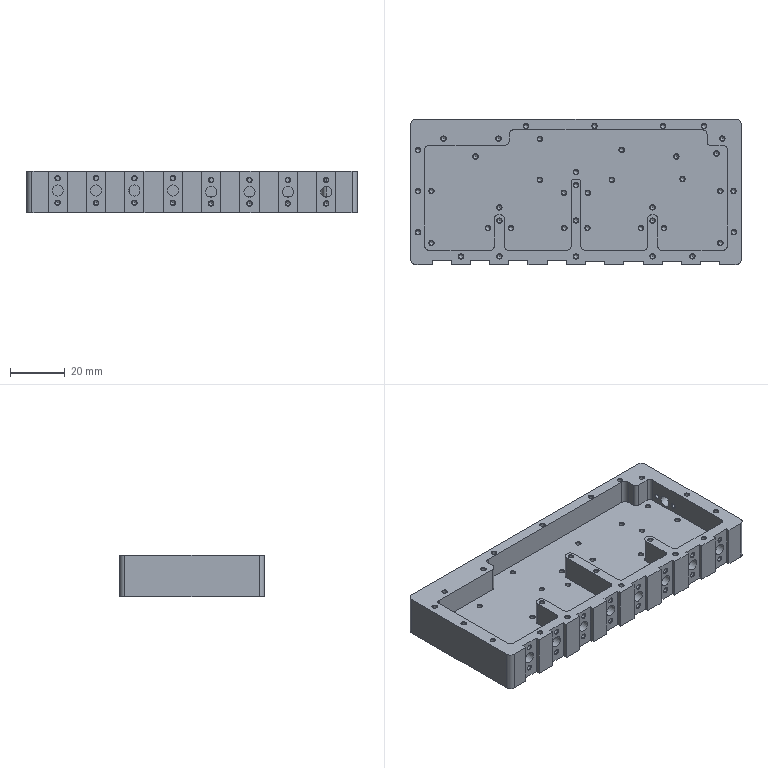Part | STEP file | 1 to 8 power divider cavity | 1 solid | 297 faces | box 120.8 x 52.94 x 15 mm | volume 53441 mm3 | cone 128 | cylinder 101 | plane 68 | commonest cylinder face diameters 1.6 x62 3 x16 4.1 x9 4 x8 2.5 x2 3.4 x2